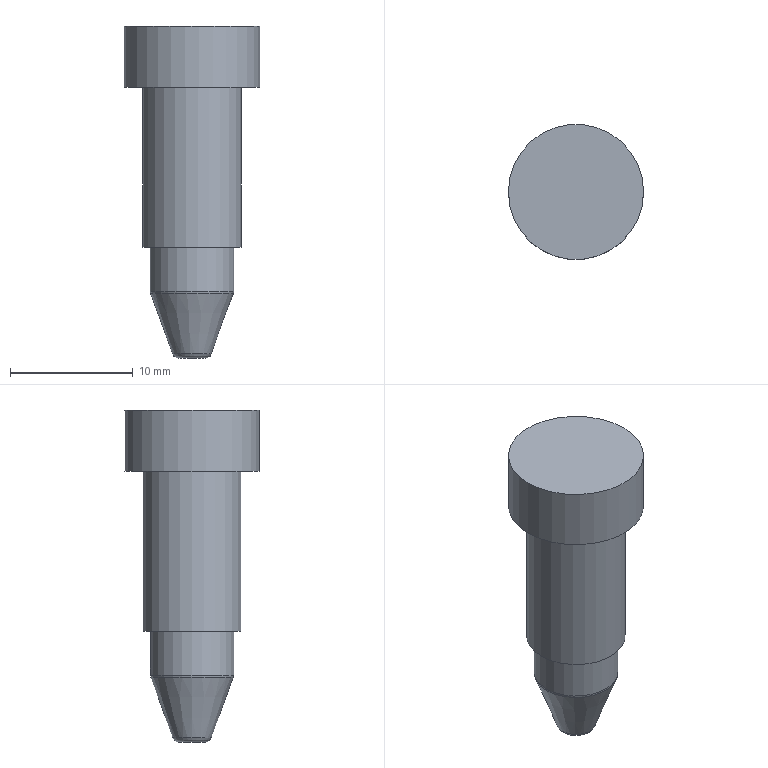Part | STEP file | gslz 2016.10.28-10_id678_x_t | 1 solid | 10 faces | box 11 x 11 x 27 mm | volume 1365 mm3 | plane 4 | cylinder 3 | torus 2 | cone 1 | commonest cylinder face diameters 6.8 x1 8 x1 11 x1
STEP:
#1=CARTESIAN_POINT('',(0.,0.,0.));
#2=DIRECTION('',(0.,0.,1.));
#3=DIRECTION('',(1.,0.,0.));
#4=AXIS2_PLACEMENT_3D('',#1,#2,#3);
#5=CARTESIAN_POINT('',(1160.2,11.,2.));
#6=VERTEX_POINT('',#5);
#7=CARTESIAN_POINT('',(1156.2,11.,2.));
#8=DIRECTION('',(0.,0.,-1.));
#9=DIRECTION('',(1.,0.,0.));
#10=AXIS2_PLACEMENT_3D('',#7,#8,#9);
#11=CIRCLE('',#10,4.);
#12=CARTESIAN_POINT('',(1156.2,11.,20.));
#13=DIRECTION('',(0.,0.,-1.));
#14=DIRECTION('',(1.,0.,0.));
#15=AXIS2_PLACEMENT_3D('',#12,#13,#14);
#16=CYLINDRICAL_SURFACE('',#15,4.);
#17=CARTESIAN_POINT('',(0.,18.));
#18=DIRECTION('',(1.,0.));
#19=VECTOR('',#18,1.);
#20=LINE('',#17,#19);
#21=(GEOMETRIC_REPRESENTATION_CONTEXT(2)PARAMETRIC_REPRESENTATION_CONTEXT()REPRESENTATION_CONTEXT('',''));
#22=DEFINITIONAL_REPRESENTATION('',(#20),#21);
#23=PCURVE('',#16,#22);
#24=CARTESIAN_POINT('',(1085.2,-19.,2.));
#25=DIRECTION('',(0.,0.,1.));
#26=DIRECTION('',(1.,0.,0.));
#27=AXIS2_PLACEMENT_3D('',#24,#25,#26);
#28=PLANE('',#27);
#29=CARTESIAN_POINT('',(75.,30.));
#30=CARTESIAN_POINT('',(75.,23.072));
#31=CARTESIAN_POINT('',(69.,26.536));
#32=CARTESIAN_POINT('',(63.,30.));
#33=CARTESIAN_POINT('',(69.,33.464));
#34=CARTESIAN_POINT('',(75.,36.928));
#35=CARTESIAN_POINT('',(75.,30.));
#36=(BOUNDED_CURVE()B_SPLINE_CURVE(2,(#29,#30,#31,#32,#33,#34,#35),.UNSPECIFIED.,.T.,.F.)B_SPLINE_CURVE_WITH_KNOTS((1,2,2,2,2,1),(-2.094,0.,2.094,4.189,6.283,8.378),.UNSPECIFIED.)CURVE()GEOMETRIC_REPRESENTATION_ITEM()RATIONAL_B_SPLINE_CURVE((1.,0.5,1.,0.5,1.,0.5,1.))REPRESENTATION_ITEM(''));
#37=(GEOMETRIC_REPRESENTATION_CONTEXT(2)PARAMETRIC_REPRESENTATION_CONTEXT()REPRESENTATION_CONTEXT('',''));
#38=DEFINITIONAL_REPRESENTATION('',(#36),#37);
#39=PCURVE('',#28,#38);
#40=SURFACE_CURVE('',#11,(#23,#39),.PCURVE_S1.);
#41=EDGE_CURVE('',#6,#6,#40,.T.);
#42=ORIENTED_EDGE('',*,*,#41,.F.);
#43=CARTESIAN_POINT('',(1160.2,11.,15.));
#44=VERTEX_POINT('',#43);
#45=CARTESIAN_POINT('',(1160.2,11.,15.));
#46=CARTESIAN_POINT('',(1160.2,11.,2.));
#47=B_SPLINE_CURVE_WITH_KNOTS('',1,(#45,#46),.UNSPECIFIED.,.F.,.F.,(2,2),(5.,18.),.PIECEWISE_BEZIER_KNOTS.);
#48=CARTESIAN_POINT('',(0.,0.));
#49=DIRECTION('',(0.,1.));
#50=VECTOR('',#49,1.);
#51=LINE('',#48,#50);
#52=(GEOMETRIC_REPRESENTATION_CONTEXT(2)PARAMETRIC_REPRESENTATION_CONTEXT()REPRESENTATION_CONTEXT('',''));
#53=DEFINITIONAL_REPRESENTATION('',(#51),#52);
#54=PCURVE('',#16,#53);
#55=CARTESIAN_POINT('',(6.283,0.));
#56=DIRECTION('',(0.,1.));
#57=VECTOR('',#56,1.);
#58=LINE('',#55,#57);
#59=(GEOMETRIC_REPRESENTATION_CONTEXT(2)PARAMETRIC_REPRESENTATION_CONTEXT()REPRESENTATION_CONTEXT('',''));
#60=DEFINITIONAL_REPRESENTATION('',(#58),#59);
#61=PCURVE('',#16,#60);
#62=SEAM_CURVE('',#47,(#54,#61),.PCURVE_S1.);
#63=EDGE_CURVE('',#44,#6,#62,.T.);
#64=ORIENTED_EDGE('',*,*,#63,.F.);
#65=CARTESIAN_POINT('',(1152.2,11.,15.));
#66=VERTEX_POINT('',#65);
#67=CARTESIAN_POINT('',(1156.2,11.,15.));
#68=DIRECTION('',(0.,0.,1.));
#69=DIRECTION('',(-1.,0.,0.));
#70=AXIS2_PLACEMENT_3D('',#67,#68,#69);
#71=CIRCLE('',#70,4.);
#72=CARTESIAN_POINT('',(3.142,5.));
#73=DIRECTION('',(-1.,0.));
#74=VECTOR('',#73,1.);
#75=LINE('',#72,#74);
#76=(GEOMETRIC_REPRESENTATION_CONTEXT(2)PARAMETRIC_REPRESENTATION_CONTEXT()REPRESENTATION_CONTEXT('',''));
#77=DEFINITIONAL_REPRESENTATION('',(#75),#76);
#78=PCURVE('',#16,#77);
#79=CARTESIAN_POINT('',(1156.2,11.,15.));
#80=DIRECTION('',(0.,0.,-1.));
#81=DIRECTION('',(1.,0.,0.));
#82=AXIS2_PLACEMENT_3D('',#79,#80,#81);
#83=PLANE('',#82);
#84=CARTESIAN_POINT('',(-4.,0.));
#85=CARTESIAN_POINT('',(-4.,6.928));
#86=CARTESIAN_POINT('',(2.,3.464));
#87=CARTESIAN_POINT('',(8.,0.));
#88=CARTESIAN_POINT('',(2.,-3.464));
#89=CARTESIAN_POINT('',(-4.,-6.928));
#90=CARTESIAN_POINT('',(-4.,0.));
#91=(BOUNDED_CURVE()B_SPLINE_CURVE(2,(#84,#85,#86,#87,#88,#89,#90),.UNSPECIFIED.,.T.,.F.)B_SPLINE_CURVE_WITH_KNOTS((1,2,2,2,2,1),(-2.094,0.,2.094,4.189,6.283,8.378),.UNSPECIFIED.)CURVE()GEOMETRIC_REPRESENTATION_ITEM()RATIONAL_B_SPLINE_CURVE((1.,0.5,1.,0.5,1.,0.5,1.))REPRESENTATION_ITEM(''));
#92=(GEOMETRIC_REPRESENTATION_CONTEXT(2)PARAMETRIC_REPRESENTATION_CONTEXT()REPRESENTATION_CONTEXT('',''));
#93=DEFINITIONAL_REPRESENTATION('',(#91),#92);
#94=PCURVE('',#83,#93);
#95=SURFACE_CURVE('',#71,(#78,#94),.PCURVE_S1.);
#96=EDGE_CURVE('',#66,#44,#95,.T.);
#97=ORIENTED_EDGE('',*,*,#96,.F.);
#98=CARTESIAN_POINT('',(1156.2,11.,15.));
#99=DIRECTION('',(0.,0.,1.));
#100=DIRECTION('',(-1.,0.,0.));
#101=AXIS2_PLACEMENT_3D('',#98,#99,#100);
#102=CIRCLE('',#101,4.);
#103=CARTESIAN_POINT('',(9.425,5.));
#104=DIRECTION('',(-1.,0.));
#105=VECTOR('',#104,1.);
#106=LINE('',#103,#105);
#107=(GEOMETRIC_REPRESENTATION_CONTEXT(2)PARAMETRIC_REPRESENTATION_CONTEXT()REPRESENTATION_CONTEXT('',''));
#108=DEFINITIONAL_REPRESENTATION('',(#106),#107);
#109=PCURVE('',#16,#108);
#110=CARTESIAN_POINT('',(-4.,0.));
#111=CARTESIAN_POINT('',(-4.,6.928));
#112=CARTESIAN_POINT('',(2.,3.464));
#113=CARTESIAN_POINT('',(8.,0.));
#114=CARTESIAN_POINT('',(2.,-3.464));
#115=CARTESIAN_POINT('',(-4.,-6.928));
#116=CARTESIAN_POINT('',(-4.,0.));
#117=(BOUNDED_CURVE()B_SPLINE_CURVE(2,(#110,#111,#112,#113,#114,#115,#116),.UNSPECIFIED.,.T.,.F.)B_SPLINE_CURVE_WITH_KNOTS((1,2,2,2,2,1),(-2.094,0.,2.094,4.189,6.283,8.378),.UNSPECIFIED.)CURVE()GEOMETRIC_REPRESENTATION_ITEM()RATIONAL_B_SPLINE_CURVE((1.,0.5,1.,0.5,1.,0.5,1.))REPRESENTATION_ITEM(''));
#118=(GEOMETRIC_REPRESENTATION_CONTEXT(2)PARAMETRIC_REPRESENTATION_CONTEXT()REPRESENTATION_CONTEXT('',''));
#119=DEFINITIONAL_REPRESENTATION('',(#117),#118);
#120=PCURVE('',#83,#119);
#121=SURFACE_CURVE('',#102,(#109,#120),.PCURVE_S1.);
#122=EDGE_CURVE('',#44,#66,#121,.T.);
#123=ORIENTED_EDGE('',*,*,#122,.F.);
#124=ORIENTED_EDGE('',*,*,#63,.T.);
#125=EDGE_LOOP('',(#42,#64,#97,#123,#124));
#126=FACE_BOUND('',#125,.T.);
#127=ADVANCED_FACE('',(#126),#16,.T.);
#128=CARTESIAN_POINT('',(1150.7,11.,15.));
#129=VERTEX_POINT('',#128);
#130=CARTESIAN_POINT('',(1161.7,11.,15.));
#131=VERTEX_POINT('',#130);
#132=CARTESIAN_POINT('',(1156.2,11.,15.));
#133=DIRECTION('',(0.,0.,-1.));
#134=DIRECTION('',(-1.,0.,0.));
#135=AXIS2_PLACEMENT_3D('',#132,#133,#134);
#136=CIRCLE('',#135,5.5);
#137=CARTESIAN_POINT('',(0.,0.));
#138=DIRECTION('',(-1.,0.));
#139=AXIS2_PLACEMENT_2D('',#137,#138);
#140=CIRCLE('',#139,5.5);
#141=(GEOMETRIC_REPRESENTATION_CONTEXT(2)PARAMETRIC_REPRESENTATION_CONTEXT()REPRESENTATION_CONTEXT('',''));
#142=DEFINITIONAL_REPRESENTATION('',(#140),#141);
#143=PCURVE('',#83,#142);
#144=CARTESIAN_POINT('',(1156.2,11.,20.));
#145=DIRECTION('',(0.,0.,-1.));
#146=DIRECTION('',(1.,0.,0.));
#147=AXIS2_PLACEMENT_3D('',#144,#145,#146);
#148=CYLINDRICAL_SURFACE('',#147,5.5);
#149=CARTESIAN_POINT('',(3.142,5.));
#150=DIRECTION('',(1.,0.));
#151=VECTOR('',#150,1.);
#152=LINE('',#149,#151);
#153=(GEOMETRIC_REPRESENTATION_CONTEXT(2)PARAMETRIC_REPRESENTATION_CONTEXT()REPRESENTATION_CONTEXT('',''));
#154=DEFINITIONAL_REPRESENTATION('',(#152),#153);
#155=PCURVE('',#148,#154);
#156=SURFACE_CURVE('',#136,(#143,#155),.PCURVE_S1.);
#157=EDGE_CURVE('',#129,#131,#156,.T.);
#158=ORIENTED_EDGE('',*,*,#157,.T.);
#159=CARTESIAN_POINT('',(1156.2,11.,15.));
#160=DIRECTION('',(0.,0.,-1.));
#161=DIRECTION('',(-1.,0.,0.));
#162=AXIS2_PLACEMENT_3D('',#159,#160,#161);
#163=CIRCLE('',#162,5.5);
#164=CARTESIAN_POINT('',(0.,0.));
#165=DIRECTION('',(-1.,0.));
#166=AXIS2_PLACEMENT_2D('',#164,#165);
#167=CIRCLE('',#166,5.5);
#168=(GEOMETRIC_REPRESENTATION_CONTEXT(2)PARAMETRIC_REPRESENTATION_CONTEXT()REPRESENTATION_CONTEXT('',''));
#169=DEFINITIONAL_REPRESENTATION('',(#167),#168);
#170=PCURVE('',#83,#169);
#171=CARTESIAN_POINT('',(-3.142,5.));
#172=DIRECTION('',(1.,0.));
#173=VECTOR('',#172,1.);
#174=LINE('',#171,#173);
#175=(GEOMETRIC_REPRESENTATION_CONTEXT(2)PARAMETRIC_REPRESENTATION_CONTEXT()REPRESENTATION_CONTEXT('',''));
#176=DEFINITIONAL_REPRESENTATION('',(#174),#175);
#177=PCURVE('',#148,#176);
#178=SURFACE_CURVE('',#163,(#170,#177),.PCURVE_S1.);
#179=EDGE_CURVE('',#131,#129,#178,.T.);
#180=ORIENTED_EDGE('',*,*,#179,.T.);
#181=EDGE_LOOP('',(#158,#180));
#182=FACE_BOUND('',#181,.T.);
#183=ORIENTED_EDGE('',*,*,#96,.T.);
#184=ORIENTED_EDGE('',*,*,#122,.T.);
#185=EDGE_LOOP('',(#183,#184));
#186=FACE_BOUND('',#185,.T.);
#187=ADVANCED_FACE('',(#182,#186),#83,.T.);
#188=CARTESIAN_POINT('',(1161.7,11.,20.));
#189=VERTEX_POINT('',#188);
#190=CARTESIAN_POINT('',(1156.2,11.,20.));
#191=DIRECTION('',(0.,0.,1.));
#192=DIRECTION('',(1.,0.,0.));
#193=AXIS2_PLACEMENT_3D('',#190,#191,#192);
#194=CIRCLE('',#193,5.5);
#195=CARTESIAN_POINT('',(1156.2,11.,20.));
#196=DIRECTION('',(0.,0.,1.));
#197=DIRECTION('',(-1.,0.,0.));
#198=AXIS2_PLACEMENT_3D('',#195,#196,#197);
#199=PLANE('',#198);
#200=CARTESIAN_POINT('',(0.,0.));
#201=DIRECTION('',(-1.,0.));
#202=AXIS2_PLACEMENT_2D('',#200,#201);
#203=CIRCLE('',#202,5.5);
#204=(GEOMETRIC_REPRESENTATION_CONTEXT(2)PARAMETRIC_REPRESENTATION_CONTEXT()REPRESENTATION_CONTEXT('',''));
#205=DEFINITIONAL_REPRESENTATION('',(#203),#204);
#206=PCURVE('',#199,#205);
#207=CARTESIAN_POINT('',(6.283,0.));
#208=DIRECTION('',(-1.,0.));
#209=VECTOR('',#208,1.);
#210=LINE('',#207,#209);
#211=(GEOMETRIC_REPRESENTATION_CONTEXT(2)PARAMETRIC_REPRESENTATION_CONTEXT()REPRESENTATION_CONTEXT('',''));
#212=DEFINITIONAL_REPRESENTATION('',(#210),#211);
#213=PCURVE('',#148,#212);
#214=SURFACE_CURVE('',#194,(#206,#213),.PCURVE_S1.);
#215=EDGE_CURVE('',#189,#189,#214,.T.);
#216=ORIENTED_EDGE('',*,*,#215,.T.);
#217=EDGE_LOOP('',(#216));
#218=FACE_BOUND('',#217,.T.);
#219=ADVANCED_FACE('',(#218),#199,.T.);
#220=ORIENTED_EDGE('',*,*,#179,.F.);
#221=CARTESIAN_POINT('',(1161.7,11.,20.));
#222=CARTESIAN_POINT('',(1161.7,11.,15.));
#223=B_SPLINE_CURVE_WITH_KNOTS('',1,(#221,#222),.UNSPECIFIED.,.F.,.F.,(2,2),(0.,5.),.PIECEWISE_BEZIER_KNOTS.);
#224=CARTESIAN_POINT('',(0.,0.));
#225=DIRECTION('',(0.,1.));
#226=VECTOR('',#225,1.);
#227=LINE('',#224,#226);
#228=(GEOMETRIC_REPRESENTATION_CONTEXT(2)PARAMETRIC_REPRESENTATION_CONTEXT()REPRESENTATION_CONTEXT('',''));
#229=DEFINITIONAL_REPRESENTATION('',(#227),#228);
#230=PCURVE('',#148,#229);
#231=CARTESIAN_POINT('',(6.283,0.));
#232=DIRECTION('',(0.,1.));
#233=VECTOR('',#232,1.);
#234=LINE('',#231,#233);
#235=(GEOMETRIC_REPRESENTATION_CONTEXT(2)PARAMETRIC_REPRESENTATION_CONTEXT()REPRESENTATION_CONTEXT('',''));
#236=DEFINITIONAL_REPRESENTATION('',(#234),#235);
#237=PCURVE('',#148,#236);
#238=SEAM_CURVE('',#223,(#230,#237),.PCURVE_S1.);
#239=EDGE_CURVE('',#189,#131,#238,.T.);
#240=ORIENTED_EDGE('',*,*,#239,.F.);
#241=ORIENTED_EDGE('',*,*,#215,.F.);
#242=ORIENTED_EDGE('',*,*,#239,.T.);
#243=ORIENTED_EDGE('',*,*,#157,.F.);
#244=EDGE_LOOP('',(#220,#240,#241,#242,#243));
#245=FACE_BOUND('',#244,.T.);
#246=ADVANCED_FACE('',(#245),#148,.T.);
#247=CARTESIAN_POINT('',(1159.6,11.,2.));
#248=VERTEX_POINT('',#247);
#249=CARTESIAN_POINT('',(1156.2,11.,2.));
#250=DIRECTION('',(0.,0.,1.));
#251=DIRECTION('',(1.,0.,0.));
#252=AXIS2_PLACEMENT_3D('',#249,#250,#251);
#253=CIRCLE('',#252,3.4);
#254=CARTESIAN_POINT('',(71.,30.));
#255=DIRECTION('',(1.,0.));
#256=AXIS2_PLACEMENT_2D('',#254,#255);
#257=CIRCLE('',#256,3.4);
#258=(GEOMETRIC_REPRESENTATION_CONTEXT(2)PARAMETRIC_REPRESENTATION_CONTEXT()REPRESENTATION_CONTEXT('',''));
#259=DEFINITIONAL_REPRESENTATION('',(#257),#258);
#260=PCURVE('',#28,#259);
#261=CARTESIAN_POINT('',(1156.2,11.,20.));
#262=DIRECTION('',(0.,0.,-1.));
#263=DIRECTION('',(1.,0.,0.));
#264=AXIS2_PLACEMENT_3D('',#261,#262,#263);
#265=CYLINDRICAL_SURFACE('',#264,3.4);
#266=CARTESIAN_POINT('',(6.283,18.));
#267=DIRECTION('',(-1.,0.));
#268=VECTOR('',#267,1.);
#269=LINE('',#266,#268);
#270=(GEOMETRIC_REPRESENTATION_CONTEXT(2)PARAMETRIC_REPRESENTATION_CONTEXT()REPRESENTATION_CONTEXT('',''));
#271=DEFINITIONAL_REPRESENTATION('',(#269),#270);
#272=PCURVE('',#265,#271);
#273=SURFACE_CURVE('',#253,(#260,#272),.PCURVE_S1.);
#274=EDGE_CURVE('',#248,#248,#273,.T.);
#275=ORIENTED_EDGE('',*,*,#274,.T.);
#276=EDGE_LOOP('',(#275));
#277=FACE_BOUND('',#276,.T.);
#278=ORIENTED_EDGE('',*,*,#41,.T.);
#279=EDGE_LOOP('',(#278));
#280=FACE_BOUND('',#279,.T.);
#281=ADVANCED_FACE('',(#277,#280),#28,.F.);
#282=CARTESIAN_POINT('',(1157.302,11.,-7.));
#283=VERTEX_POINT('',#282);
#284=CARTESIAN_POINT('',(1156.2,11.,-7.));
#285=DIRECTION('',(0.,0.,-1.));
#286=DIRECTION('',(1.,0.,0.));
#287=AXIS2_PLACEMENT_3D('',#284,#285,#286);
#288=CIRCLE('',#287,1.102);
#289=CARTESIAN_POINT('',(1086.5,-3.,-7.));
#290=DIRECTION('',(0.,0.,1.));
#291=DIRECTION('',(-1.,0.,0.));
#292=AXIS2_PLACEMENT_3D('',#289,#290,#291);
#293=PLANE('',#292);
#294=CARTESIAN_POINT('',(-70.802,-14.));
#295=CARTESIAN_POINT('',(-70.802,-12.091));
#296=CARTESIAN_POINT('',(-69.149,-13.046));
#297=CARTESIAN_POINT('',(-67.496,-14.));
#298=CARTESIAN_POINT('',(-69.149,-14.954));
#299=CARTESIAN_POINT('',(-70.802,-15.909));
#300=CARTESIAN_POINT('',(-70.802,-14.));
#301=(BOUNDED_CURVE()B_SPLINE_CURVE(2,(#294,#295,#296,#297,#298,#299,#300),.UNSPECIFIED.,.T.,.F.)B_SPLINE_CURVE_WITH_KNOTS((1,2,2,2,2,1),(-2.094,0.,2.094,4.189,6.283,8.378),.UNSPECIFIED.)CURVE()GEOMETRIC_REPRESENTATION_ITEM()RATIONAL_B_SPLINE_CURVE((1.,0.5,1.,0.5,1.,0.5,1.))REPRESENTATION_ITEM(''));
#302=(GEOMETRIC_REPRESENTATION_CONTEXT(2)PARAMETRIC_REPRESENTATION_CONTEXT()REPRESENTATION_CONTEXT('',''));
#303=DEFINITIONAL_REPRESENTATION('',(#301),#302);
#304=PCURVE('',#293,#303);
#305=CARTESIAN_POINT('',(1156.2,11.,-6.5));
#306=DIRECTION('',(0.,0.,1.));
#307=DIRECTION('',(1.,0.,0.));
#308=AXIS2_PLACEMENT_3D('',#305,#306,#307);
#309=TOROIDAL_SURFACE('',#308,1.102,0.5);
#310=CARTESIAN_POINT('',(6.283,4.712));
#311=DIRECTION('',(-1.,0.));
#312=VECTOR('',#311,1.);
#313=LINE('',#310,#312);
#314=(GEOMETRIC_REPRESENTATION_CONTEXT(2)PARAMETRIC_REPRESENTATION_CONTEXT()REPRESENTATION_CONTEXT('',''));
#315=DEFINITIONAL_REPRESENTATION('',(#313),#314);
#316=PCURVE('',#309,#315);
#317=SURFACE_CURVE('',#288,(#304,#316),.PCURVE_S1.);
#318=EDGE_CURVE('',#283,#283,#317,.T.);
#319=ORIENTED_EDGE('',*,*,#318,.T.);
#320=EDGE_LOOP('',(#319));
#321=FACE_BOUND('',#320,.T.);
#322=ADVANCED_FACE('',(#321),#293,.F.);
#323=CARTESIAN_POINT('',(1154.628,11.,-6.671));
#324=VERTEX_POINT('',#323);
#325=CARTESIAN_POINT('',(1157.772,11.,-6.671));
#326=VERTEX_POINT('',#325);
#327=CARTESIAN_POINT('',(1156.2,11.,-6.671));
#328=DIRECTION('',(0.,0.,1.));
#329=DIRECTION('',(-1.,0.,0.));
#330=AXIS2_PLACEMENT_3D('',#327,#328,#329);
#331=CIRCLE('',#330,1.572);
#332=CARTESIAN_POINT('',(1156.2,11.,0.));
#333=DIRECTION('',(0.,0.,1.));
#334=DIRECTION('',(-1.,0.,0.));
#335=AXIS2_PLACEMENT_3D('',#332,#333,#334);
#336=CONICAL_SURFACE('',#335,4.,0.3491);
#337=CARTESIAN_POINT('',(0.,-6.671));
#338=DIRECTION('',(1.,0.));
#339=VECTOR('',#338,1.);
#340=LINE('',#337,#339);
#341=(GEOMETRIC_REPRESENTATION_CONTEXT(2)PARAMETRIC_REPRESENTATION_CONTEXT()REPRESENTATION_CONTEXT('',''));
#342=DEFINITIONAL_REPRESENTATION('',(#340),#341);
#343=PCURVE('',#336,#342);
#344=CARTESIAN_POINT('',(3.142,5.934));
#345=DIRECTION('',(1.,0.));
#346=VECTOR('',#345,1.);
#347=LINE('',#344,#346);
#348=(GEOMETRIC_REPRESENTATION_CONTEXT(2)PARAMETRIC_REPRESENTATION_CONTEXT()REPRESENTATION_CONTEXT('',''));
#349=DEFINITIONAL_REPRESENTATION('',(#347),#348);
#350=PCURVE('',#309,#349);
#351=SURFACE_CURVE('',#331,(#343,#350),.PCURVE_S1.);
#352=EDGE_CURVE('',#324,#326,#351,.T.);
#353=ORIENTED_EDGE('',*,*,#352,.T.);
#354=CARTESIAN_POINT('',(1156.2,11.,-6.671));
#355=DIRECTION('',(0.,0.,1.));
#356=DIRECTION('',(-1.,0.,0.));
#357=AXIS2_PLACEMENT_3D('',#354,#355,#356);
#358=CIRCLE('',#357,1.572);
#359=CARTESIAN_POINT('',(0.,-6.671));
#360=DIRECTION('',(1.,0.));
#361=VECTOR('',#360,1.);
#362=LINE('',#359,#361);
#363=(GEOMETRIC_REPRESENTATION_CONTEXT(2)PARAMETRIC_REPRESENTATION_CONTEXT()REPRESENTATION_CONTEXT('',''));
#364=DEFINITIONAL_REPRESENTATION('',(#362),#363);
#365=PCURVE('',#336,#364);
#366=CARTESIAN_POINT('',(-3.142,5.934));
#367=DIRECTION('',(1.,0.));
#368=VECTOR('',#367,1.);
#369=LINE('',#366,#368);
#370=(GEOMETRIC_REPRESENTATION_CONTEXT(2)PARAMETRIC_REPRESENTATION_CONTEXT()REPRESENTATION_CONTEXT('',''));
#371=DEFINITIONAL_REPRESENTATION('',(#369),#370);
#372=PCURVE('',#309,#371);
#373=SURFACE_CURVE('',#358,(#365,#372),.PCURVE_S1.);
#374=EDGE_CURVE('',#326,#324,#373,.T.);
#375=ORIENTED_EDGE('',*,*,#374,.T.);
#376=CARTESIAN_POINT('',(1152.83,11.,-1.731));
#377=VERTEX_POINT('',#376);
#378=CARTESIAN_POINT('',(1154.628,11.,-6.671));
#379=CARTESIAN_POINT('',(1152.83,11.,-1.731));
#380=B_SPLINE_CURVE_WITH_KNOTS('',1,(#378,#379),.UNSPECIFIED.,.F.,.F.,(2,2),(-7.099,-1.842),.PIECEWISE_BEZIER_KNOTS.);
#381=CARTESIAN_POINT('',(6.283,0.));
#382=DIRECTION('',(0.,1.));
#383=VECTOR('',#382,1.);
#384=LINE('',#381,#383);
#385=(GEOMETRIC_REPRESENTATION_CONTEXT(2)PARAMETRIC_REPRESENTATION_CONTEXT()REPRESENTATION_CONTEXT('',''));
#386=DEFINITIONAL_REPRESENTATION('',(#384),#385);
#387=PCURVE('',#336,#386);
#388=CARTESIAN_POINT('',(0.,0.));
#389=DIRECTION('',(0.,1.));
#390=VECTOR('',#389,1.);
#391=LINE('',#388,#390);
#392=(GEOMETRIC_REPRESENTATION_CONTEXT(2)PARAMETRIC_REPRESENTATION_CONTEXT()REPRESENTATION_CONTEXT('',''));
#393=DEFINITIONAL_REPRESENTATION('',(#391),#392);
#394=PCURVE('',#336,#393);
#395=SEAM_CURVE('',#380,(#387,#394),.PCURVE_S1.);
#396=EDGE_CURVE('',#324,#377,#395,.T.);
#397=ORIENTED_EDGE('',*,*,#396,.T.);
#398=CARTESIAN_POINT('',(1156.2,11.,-1.731));
#399=DIRECTION('',(0.,0.,-1.));
#400=DIRECTION('',(-1.,0.,0.));
#401=AXIS2_PLACEMENT_3D('',#398,#399,#400);
#402=CIRCLE('',#401,3.37);
#403=CARTESIAN_POINT('',(6.283,-1.731));
#404=DIRECTION('',(-1.,0.));
#405=VECTOR('',#404,1.);
#406=LINE('',#403,#405);
#407=(GEOMETRIC_REPRESENTATION_CONTEXT(2)PARAMETRIC_REPRESENTATION_CONTEXT()REPRESENTATION_CONTEXT('',''));
#408=DEFINITIONAL_REPRESENTATION('',(#406),#407);
#409=PCURVE('',#336,#408);
#410=CARTESIAN_POINT('',(1156.2,11.,-1.56));
#411=DIRECTION('',(0.,0.,-1.));
#412=DIRECTION('',(-1.,0.,0.));
#413=AXIS2_PLACEMENT_3D('',#410,#411,#412);
#414=TOROIDAL_SURFACE('',#413,2.9,0.5);
#415=CARTESIAN_POINT('',(0.,6.632));
#416=DIRECTION('',(1.,0.));
#417=VECTOR('',#416,1.);
#418=LINE('',#415,#417);
#419=(GEOMETRIC_REPRESENTATION_CONTEXT(2)PARAMETRIC_REPRESENTATION_CONTEXT()REPRESENTATION_CONTEXT('',''));
#420=DEFINITIONAL_REPRESENTATION('',(#418),#419);
#421=PCURVE('',#414,#420);
#422=SURFACE_CURVE('',#402,(#409,#421),.PCURVE_S1.);
#423=EDGE_CURVE('',#377,#377,#422,.T.);
#424=ORIENTED_EDGE('',*,*,#423,.T.);
#425=ORIENTED_EDGE('',*,*,#396,.F.);
#426=EDGE_LOOP('',(#353,#375,#397,#424,#425));
#427=FACE_BOUND('',#426,.T.);
#428=ADVANCED_FACE('',(#427),#336,.T.);
#429=CARTESIAN_POINT('',(1152.8,11.,-1.56));
#430=VERTEX_POINT('',#429);
#431=CARTESIAN_POINT('',(1159.6,11.,-1.56));
#432=VERTEX_POINT('',#431);
#433=CARTESIAN_POINT('',(1156.2,11.,-1.56));
#434=DIRECTION('',(0.,0.,1.));
#435=DIRECTION('',(-1.,0.,0.));
#436=AXIS2_PLACEMENT_3D('',#433,#434,#435);
#437=CIRCLE('',#436,3.4);
#438=CARTESIAN_POINT('',(3.142,21.56));
#439=DIRECTION('',(-1.,0.));
#440=VECTOR('',#439,1.);
#441=LINE('',#438,#440);
#442=(GEOMETRIC_REPRESENTATION_CONTEXT(2)PARAMETRIC_REPRESENTATION_CONTEXT()REPRESENTATION_CONTEXT('',''));
#443=DEFINITIONAL_REPRESENTATION('',(#441),#442);
#444=PCURVE('',#265,#443);
#445=CARTESIAN_POINT('',(6.283,6.283));
#446=DIRECTION('',(-1.,0.));
#447=VECTOR('',#446,1.);
#448=LINE('',#445,#447);
#449=(GEOMETRIC_REPRESENTATION_CONTEXT(2)PARAMETRIC_REPRESENTATION_CONTEXT()REPRESENTATION_CONTEXT('',''));
#450=DEFINITIONAL_REPRESENTATION('',(#448),#449);
#451=PCURVE('',#414,#450);
#452=SURFACE_CURVE('',#437,(#444,#451),.PCURVE_S1.);
#453=EDGE_CURVE('',#430,#432,#452,.T.);
#454=ORIENTED_EDGE('',*,*,#453,.T.);
#455=CARTESIAN_POINT('',(1159.6,11.,2.));
#456=CARTESIAN_POINT('',(1159.6,11.,-1.56));
#457=B_SPLINE_CURVE_WITH_KNOTS('',1,(#455,#456),.UNSPECIFIED.,.F.,.F.,(2,2),(18.,21.56),.PIECEWISE_BEZIER_KNOTS.);
#458=CARTESIAN_POINT('',(0.,0.));
#459=DIRECTION('',(0.,1.));
#460=VECTOR('',#459,1.);
#461=LINE('',#458,#460);
#462=(GEOMETRIC_REPRESENTATION_CONTEXT(2)PARAMETRIC_REPRESENTATION_CONTEXT()REPRESENTATION_CONTEXT('',''));
#463=DEFINITIONAL_REPRESENTATION('',(#461),#462);
#464=PCURVE('',#265,#463);
#465=CARTESIAN_POINT('',(6.283,0.));
#466=DIRECTION('',(0.,1.));
#467=VECTOR('',#466,1.);
#468=LINE('',#465,#467);
#469=(GEOMETRIC_REPRESENTATION_CONTEXT(2)PARAMETRIC_REPRESENTATION_CONTEXT()REPRESENTATION_CONTEXT('',''));
#470=DEFINITIONAL_REPRESENTATION('',(#468),#469);
#471=PCURVE('',#265,#470);
#472=SEAM_CURVE('',#457,(#464,#471),.PCURVE_S1.);
#473=EDGE_CURVE('',#248,#432,#472,.T.);
#474=ORIENTED_EDGE('',*,*,#473,.F.);
#475=ORIENTED_EDGE('',*,*,#274,.F.);
#476=ORIENTED_EDGE('',*,*,#473,.T.);
#477=CARTESIAN_POINT('',(1156.2,11.,-1.56));
#478=DIRECTION('',(0.,0.,1.));
#479=DIRECTION('',(-1.,0.,0.));
#480=AXIS2_PLACEMENT_3D('',#477,#478,#479);
#481=CIRCLE('',#480,3.4);
#482=CARTESIAN_POINT('',(9.425,21.56));
#483=DIRECTION('',(-1.,0.));
#484=VECTOR('',#483,1.);
#485=LINE('',#482,#484);
#486=(GEOMETRIC_REPRESENTATION_CONTEXT(2)PARAMETRIC_REPRESENTATION_CONTEXT()REPRESENTATION_CONTEXT('',''));
#487=DEFINITIONAL_REPRESENTATION('',(#485),#486);
#488=PCURVE('',#265,#487);
#489=CARTESIAN_POINT('',(6.283,6.283));
#490=DIRECTION('',(-1.,0.));
#491=VECTOR('',#490,1.);
#492=LINE('',#489,#491);
#493=(GEOMETRIC_REPRESENTATION_CONTEXT(2)PARAMETRIC_REPRESENTATION_CONTEXT()REPRESENTATION_CONTEXT('',''));
#494=DEFINITIONAL_REPRESENTATION('',(#492),#493);
#495=PCURVE('',#414,#494);
#496=SURFACE_CURVE('',#481,(#488,#495),.PCURVE_S1.);
#497=EDGE_CURVE('',#432,#430,#496,.T.);
#498=ORIENTED_EDGE('',*,*,#497,.T.);
#499=EDGE_LOOP('',(#454,#474,#475,#476,#498));
#500=FACE_BOUND('',#499,.T.);
#501=ADVANCED_FACE('',(#500),#265,.T.);
#502=ORIENTED_EDGE('',*,*,#453,.F.);
#503=CARTESIAN_POINT('',(1152.8,11.,-1.56));
#504=CARTESIAN_POINT('',(1152.8,11.,-1.589));
#505=CARTESIAN_POINT('',(1152.802,11.,-1.619));
#506=CARTESIAN_POINT('',(1152.806,11.,-1.647));
#507=CARTESIAN_POINT('',(1152.812,11.,-1.676));
#508=CARTESIAN_POINT('',(1152.82,11.,-1.704));
#509=CARTESIAN_POINT('',(1152.83,11.,-1.731));
#510=(BOUNDED_CURVE()B_SPLINE_CURVE(6,(#503,#504,#505,#506,#507,#508,#509),.UNSPECIFIED.,.F.,.F.)B_SPLINE_CURVE_WITH_KNOTS((7,7),(0.,0.3491),.PIECEWISE_BEZIER_KNOTS.)CURVE()GEOMETRIC_REPRESENTATION_ITEM()RATIONAL_B_SPLINE_CURVE((1.002,1.001,0.9999,0.9997,0.9999,1.001,1.002))REPRESENTATION_ITEM(''));
#511=CARTESIAN_POINT('',(6.283,6.283));
#512=DIRECTION('',(0.,1.));
#513=VECTOR('',#512,1.);
#514=LINE('',#511,#513);
#515=(GEOMETRIC_REPRESENTATION_CONTEXT(2)PARAMETRIC_REPRESENTATION_CONTEXT()REPRESENTATION_CONTEXT('',''));
#516=DEFINITIONAL_REPRESENTATION('',(#514),#515);
#517=PCURVE('',#414,#516);
#518=CARTESIAN_POINT('',(0.,6.283));
#519=DIRECTION('',(0.,1.));
#520=VECTOR('',#519,1.);
#521=LINE('',#518,#520);
#522=(GEOMETRIC_REPRESENTATION_CONTEXT(2)PARAMETRIC_REPRESENTATION_CONTEXT()REPRESENTATION_CONTEXT('',''));
#523=DEFINITIONAL_REPRESENTATION('',(#521),#522);
#524=PCURVE('',#414,#523);
#525=SEAM_CURVE('',#510,(#517,#524),.PCURVE_S1.);
#526=EDGE_CURVE('',#430,#377,#525,.T.);
#527=ORIENTED_EDGE('',*,*,#526,.T.);
#528=ORIENTED_EDGE('',*,*,#423,.F.);
#529=ORIENTED_EDGE('',*,*,#526,.F.);
#530=ORIENTED_EDGE('',*,*,#497,.F.);
#531=EDGE_LOOP('',(#502,#527,#528,#529,#530));
#532=FACE_BOUND('',#531,.T.);
#533=ADVANCED_FACE('',(#532),#414,.T.);
#534=ORIENTED_EDGE('',*,*,#318,.F.);
#535=CARTESIAN_POINT('',(1157.302,11.,-7.));
#536=CARTESIAN_POINT('',(1157.405,11.,-7.));
#537=CARTESIAN_POINT('',(1157.507,11.,-6.975));
#538=CARTESIAN_POINT('',(1157.6,11.,-6.925));
#539=CARTESIAN_POINT('',(1157.678,11.,-6.855));
#540=CARTESIAN_POINT('',(1157.737,11.,-6.768));
#541=CARTESIAN_POINT('',(1157.772,11.,-6.671));
#542=(BOUNDED_CURVE()B_SPLINE_CURVE(6,(#535,#536,#537,#538,#539,#540,#541),.UNSPECIFIED.,.F.,.F.)B_SPLINE_CURVE_WITH_KNOTS((7,7),(4.712,5.934),.PIECEWISE_BEZIER_KNOTS.)CURVE()GEOMETRIC_REPRESENTATION_ITEM()RATIONAL_B_SPLINE_CURVE((1.019,1.006,0.9987,0.9963,0.9987,1.006,1.019))REPRESENTATION_ITEM(''));
#543=CARTESIAN_POINT('',(6.283,0.));
#544=DIRECTION('',(0.,1.));
#545=VECTOR('',#544,1.);
#546=LINE('',#543,#545);
#547=(GEOMETRIC_REPRESENTATION_CONTEXT(2)PARAMETRIC_REPRESENTATION_CONTEXT()REPRESENTATION_CONTEXT('',''));
#548=DEFINITIONAL_REPRESENTATION('',(#546),#547);
#549=PCURVE('',#309,#548);
#550=CARTESIAN_POINT('',(0.,0.));
#551=DIRECTION('',(0.,1.));
#552=VECTOR('',#551,1.);
#553=LINE('',#550,#552);
#554=(GEOMETRIC_REPRESENTATION_CONTEXT(2)PARAMETRIC_REPRESENTATION_CONTEXT()REPRESENTATION_CONTEXT('',''));
#555=DEFINITIONAL_REPRESENTATION('',(#553),#554);
#556=PCURVE('',#309,#555);
#557=SEAM_CURVE('',#542,(#549,#556),.PCURVE_S1.);
#558=EDGE_CURVE('',#283,#326,#557,.T.);
#559=ORIENTED_EDGE('',*,*,#558,.T.);
#560=ORIENTED_EDGE('',*,*,#352,.F.);
#561=ORIENTED_EDGE('',*,*,#374,.F.);
#562=ORIENTED_EDGE('',*,*,#558,.F.);
#563=EDGE_LOOP('',(#534,#559,#560,#561,#562));
#564=FACE_BOUND('',#563,.T.);
#565=ADVANCED_FACE('',(#564),#309,.T.);
#566=CLOSED_SHELL('',(#127,#187,#219,#246,#281,#322,#428,#501,#533,#565));
#567=MANIFOLD_SOLID_BREP('',#566);
#568=(LENGTH_UNIT()NAMED_UNIT(*)SI_UNIT(.MILLI.,.METRE.));
#569=UNCERTAINTY_MEASURE_WITH_UNIT(LENGTH_MEASURE(0.000005),#568,'','');
#570=(NAMED_UNIT(*)PLANE_ANGLE_UNIT()SI_UNIT($,.RADIAN.));
#571=(NAMED_UNIT(*)SI_UNIT($,.STERADIAN.)SOLID_ANGLE_UNIT());
#572=(GEOMETRIC_REPRESENTATION_CONTEXT(3)GLOBAL_UNCERTAINTY_ASSIGNED_CONTEXT((#569))GLOBAL_UNIT_ASSIGNED_CONTEXT((#568,#570,#571))REPRESENTATION_CONTEXT('',''));
#573=ADVANCED_BREP_SHAPE_REPRESENTATION('',(#4,#567),#572);